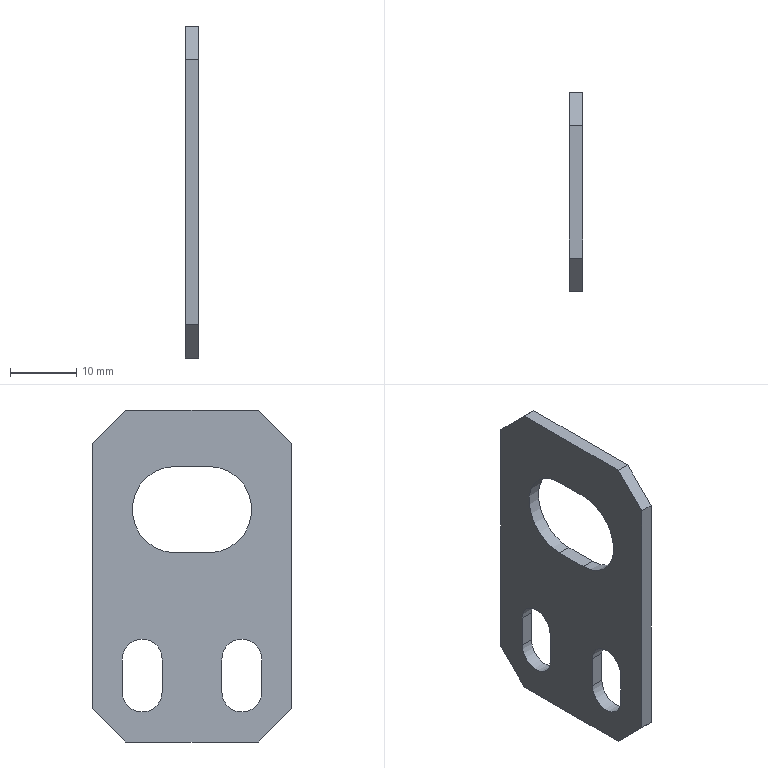Part | NX | features 5003_222_Bracket 2 | 1 solid | 22 faces | box 2 x 30 x 50 mm | volume 2271 mm3 | plane 16 | cylinder 6 | commonest cylinder face diameters 6 x4 13 x2
STEP:
#1=CARTESIAN_POINT('',(218.525,88.5,-44.5));
#2=VERTEX_POINT('',#1);
#3=CARTESIAN_POINT('',(218.525,88.5,-49.5));
#4=VERTEX_POINT('',#3);
#5=CARTESIAN_POINT('',(218.525,88.5,-44.5));
#6=DIRECTION('',(0.,0.,-1.));
#7=VECTOR('',#6,1000.);
#8=LINE('',#5,#7);
#9=EDGE_CURVE('',#2,#4,#8,.T.);
#10=ORIENTED_EDGE('',*,*,#9,.F.);
#11=CARTESIAN_POINT('',(218.525,82.5,-44.5));
#12=VERTEX_POINT('',#11);
#13=CARTESIAN_POINT('',(218.525,85.5,-44.5));
#14=DIRECTION('',(-1.,0.,0.));
#15=DIRECTION('',(0.,0.,-1.));
#16=AXIS2_PLACEMENT_3D('',#13,#14,#15);
#17=CIRCLE('',#16,3.);
#18=EDGE_CURVE('',#12,#2,#17,.T.);
#19=ORIENTED_EDGE('',*,*,#18,.F.);
#20=CARTESIAN_POINT('',(218.525,82.5,-49.5));
#21=VERTEX_POINT('',#20);
#22=CARTESIAN_POINT('',(218.525,82.5,-44.5));
#23=DIRECTION('',(0.,0.,1.));
#24=VECTOR('',#23,1000.);
#25=LINE('',#22,#24);
#26=EDGE_CURVE('',#21,#12,#25,.T.);
#27=ORIENTED_EDGE('',*,*,#26,.F.);
#28=CARTESIAN_POINT('',(218.525,85.5,-49.5));
#29=DIRECTION('',(-1.,0.,0.));
#30=DIRECTION('',(0.,0.,-1.));
#31=AXIS2_PLACEMENT_3D('',#28,#29,#30);
#32=CIRCLE('',#31,3.);
#33=EDGE_CURVE('',#4,#21,#32,.T.);
#34=ORIENTED_EDGE('',*,*,#33,.F.);
#35=EDGE_LOOP('',(#10,#19,#27,#34));
#36=FACE_BOUND('',#35,.T.);
#37=CARTESIAN_POINT('',(218.525,78.,-52.));
#38=VERTEX_POINT('',#37);
#39=CARTESIAN_POINT('',(218.525,78.,-12.));
#40=VERTEX_POINT('',#39);
#41=CARTESIAN_POINT('',(218.525,78.,-52.));
#42=DIRECTION('',(0.,0.,1.));
#43=VECTOR('',#42,1000.);
#44=LINE('',#41,#43);
#45=EDGE_CURVE('',#38,#40,#44,.T.);
#46=ORIENTED_EDGE('',*,*,#45,.T.);
#47=CARTESIAN_POINT('',(218.525,83.,-7.));
#48=VERTEX_POINT('',#47);
#49=CARTESIAN_POINT('',(218.525,78.,-12.));
#50=DIRECTION('',(0.,0.7071,0.7071));
#51=VECTOR('',#50,1000.);
#52=LINE('',#49,#51);
#53=EDGE_CURVE('',#40,#48,#52,.T.);
#54=ORIENTED_EDGE('',*,*,#53,.T.);
#55=CARTESIAN_POINT('',(218.525,103.,-7.));
#56=VERTEX_POINT('',#55);
#57=CARTESIAN_POINT('',(218.525,83.,-7.));
#58=DIRECTION('',(0.,1.,0.));
#59=VECTOR('',#58,1000.);
#60=LINE('',#57,#59);
#61=EDGE_CURVE('',#48,#56,#60,.T.);
#62=ORIENTED_EDGE('',*,*,#61,.T.);
#63=CARTESIAN_POINT('',(218.525,108.,-12.));
#64=VERTEX_POINT('',#63);
#65=CARTESIAN_POINT('',(218.525,103.,-7.));
#66=DIRECTION('',(0.,0.7071,-0.7071));
#67=VECTOR('',#66,1000.);
#68=LINE('',#65,#67);
#69=EDGE_CURVE('',#56,#64,#68,.T.);
#70=ORIENTED_EDGE('',*,*,#69,.T.);
#71=CARTESIAN_POINT('',(218.525,108.,-52.));
#72=VERTEX_POINT('',#71);
#73=CARTESIAN_POINT('',(218.525,108.,-12.));
#74=DIRECTION('',(0.,0.,-1.));
#75=VECTOR('',#74,1000.);
#76=LINE('',#73,#75);
#77=EDGE_CURVE('',#64,#72,#76,.T.);
#78=ORIENTED_EDGE('',*,*,#77,.T.);
#79=CARTESIAN_POINT('',(218.525,103.,-57.));
#80=VERTEX_POINT('',#79);
#81=CARTESIAN_POINT('',(218.525,108.,-52.));
#82=DIRECTION('',(0.,-0.7071,-0.7071));
#83=VECTOR('',#82,1000.);
#84=LINE('',#81,#83);
#85=EDGE_CURVE('',#72,#80,#84,.T.);
#86=ORIENTED_EDGE('',*,*,#85,.T.);
#87=CARTESIAN_POINT('',(218.525,83.,-57.));
#88=VERTEX_POINT('',#87);
#89=CARTESIAN_POINT('',(218.525,103.,-57.));
#90=DIRECTION('',(0.,-1.,0.));
#91=VECTOR('',#90,1000.);
#92=LINE('',#89,#91);
#93=EDGE_CURVE('',#80,#88,#92,.T.);
#94=ORIENTED_EDGE('',*,*,#93,.T.);
#95=CARTESIAN_POINT('',(218.525,83.,-57.));
#96=DIRECTION('',(0.,-0.7071,0.7071));
#97=VECTOR('',#96,1000.);
#98=LINE('',#95,#97);
#99=EDGE_CURVE('',#88,#38,#98,.T.);
#100=ORIENTED_EDGE('',*,*,#99,.T.);
#101=EDGE_LOOP('',(#46,#54,#62,#70,#78,#86,#94,#100));
#102=FACE_BOUND('',#101,.T.);
#103=CARTESIAN_POINT('',(218.525,90.5,-15.5));
#104=VERTEX_POINT('',#103);
#105=CARTESIAN_POINT('',(218.525,95.5,-15.5));
#106=VERTEX_POINT('',#105);
#107=CARTESIAN_POINT('',(218.525,90.5,-15.5));
#108=DIRECTION('',(0.,1.,0.));
#109=VECTOR('',#108,1000.);
#110=LINE('',#107,#109);
#111=EDGE_CURVE('',#104,#106,#110,.T.);
#112=ORIENTED_EDGE('',*,*,#111,.F.);
#113=CARTESIAN_POINT('',(218.525,90.5,-28.5));
#114=VERTEX_POINT('',#113);
#115=CARTESIAN_POINT('',(218.525,90.5,-22.));
#116=DIRECTION('',(-1.,0.,0.));
#117=DIRECTION('',(0.,0.,-1.));
#118=AXIS2_PLACEMENT_3D('',#115,#116,#117);
#119=CIRCLE('',#118,6.5);
#120=EDGE_CURVE('',#114,#104,#119,.T.);
#121=ORIENTED_EDGE('',*,*,#120,.F.);
#122=CARTESIAN_POINT('',(218.525,95.5,-28.5));
#123=VERTEX_POINT('',#122);
#124=CARTESIAN_POINT('',(218.525,90.5,-28.5));
#125=DIRECTION('',(0.,-1.,0.));
#126=VECTOR('',#125,1000.);
#127=LINE('',#124,#126);
#128=EDGE_CURVE('',#123,#114,#127,.T.);
#129=ORIENTED_EDGE('',*,*,#128,.F.);
#130=CARTESIAN_POINT('',(218.525,95.5,-22.));
#131=DIRECTION('',(-1.,0.,0.));
#132=DIRECTION('',(0.,0.,-1.));
#133=AXIS2_PLACEMENT_3D('',#130,#131,#132);
#134=CIRCLE('',#133,6.5);
#135=EDGE_CURVE('',#106,#123,#134,.T.);
#136=ORIENTED_EDGE('',*,*,#135,.F.);
#137=EDGE_LOOP('',(#112,#121,#129,#136));
#138=FACE_BOUND('',#137,.T.);
#139=CARTESIAN_POINT('',(218.525,97.5,-49.5));
#140=VERTEX_POINT('',#139);
#141=CARTESIAN_POINT('',(218.525,97.5,-44.5));
#142=VERTEX_POINT('',#141);
#143=CARTESIAN_POINT('',(218.525,97.5,-44.5));
#144=DIRECTION('',(0.,0.,1.));
#145=VECTOR('',#144,1000.);
#146=LINE('',#143,#145);
#147=EDGE_CURVE('',#140,#142,#146,.T.);
#148=ORIENTED_EDGE('',*,*,#147,.F.);
#149=CARTESIAN_POINT('',(218.525,103.5,-49.5));
#150=VERTEX_POINT('',#149);
#151=CARTESIAN_POINT('',(218.525,100.5,-49.5));
#152=DIRECTION('',(-1.,0.,0.));
#153=DIRECTION('',(0.,0.,-1.));
#154=AXIS2_PLACEMENT_3D('',#151,#152,#153);
#155=CIRCLE('',#154,3.);
#156=EDGE_CURVE('',#150,#140,#155,.T.);
#157=ORIENTED_EDGE('',*,*,#156,.F.);
#158=CARTESIAN_POINT('',(218.525,103.5,-44.5));
#159=VERTEX_POINT('',#158);
#160=CARTESIAN_POINT('',(218.525,103.5,-44.5));
#161=DIRECTION('',(0.,0.,-1.));
#162=VECTOR('',#161,1000.);
#163=LINE('',#160,#162);
#164=EDGE_CURVE('',#159,#150,#163,.T.);
#165=ORIENTED_EDGE('',*,*,#164,.F.);
#166=CARTESIAN_POINT('',(218.525,100.5,-44.5));
#167=DIRECTION('',(-1.,0.,0.));
#168=DIRECTION('',(0.,0.,-1.));
#169=AXIS2_PLACEMENT_3D('',#166,#167,#168);
#170=CIRCLE('',#169,3.);
#171=EDGE_CURVE('',#142,#159,#170,.T.);
#172=ORIENTED_EDGE('',*,*,#171,.F.);
#173=EDGE_LOOP('',(#148,#157,#165,#172));
#174=FACE_BOUND('',#173,.T.);
#175=CARTESIAN_POINT('',(218.525,108.,-32.));
#176=DIRECTION('',(-1.,0.,0.));
#177=DIRECTION('',(0.,0.,-1.));
#178=AXIS2_PLACEMENT_3D('',#175,#176,#177);
#179=PLANE('',#178);
#180=ADVANCED_FACE('',(#36,#102,#138,#174),#179,.T.);
#181=CARTESIAN_POINT('',(220.525,82.5,-44.5));
#182=VERTEX_POINT('',#181);
#183=CARTESIAN_POINT('',(220.525,88.5,-44.5));
#184=VERTEX_POINT('',#183);
#185=CARTESIAN_POINT('',(220.525,85.5,-44.5));
#186=DIRECTION('',(-1.,0.,0.));
#187=DIRECTION('',(0.,0.,-1.));
#188=AXIS2_PLACEMENT_3D('',#185,#186,#187);
#189=CIRCLE('',#188,3.);
#190=EDGE_CURVE('',#182,#184,#189,.T.);
#191=ORIENTED_EDGE('',*,*,#190,.T.);
#192=CARTESIAN_POINT('',(220.525,88.5,-49.5));
#193=VERTEX_POINT('',#192);
#194=CARTESIAN_POINT('',(220.525,88.5,-44.5));
#195=DIRECTION('',(0.,0.,-1.));
#196=VECTOR('',#195,1000.);
#197=LINE('',#194,#196);
#198=EDGE_CURVE('',#184,#193,#197,.T.);
#199=ORIENTED_EDGE('',*,*,#198,.T.);
#200=CARTESIAN_POINT('',(220.525,82.5,-49.5));
#201=VERTEX_POINT('',#200);
#202=CARTESIAN_POINT('',(220.525,85.5,-49.5));
#203=DIRECTION('',(-1.,0.,0.));
#204=DIRECTION('',(0.,0.,-1.));
#205=AXIS2_PLACEMENT_3D('',#202,#203,#204);
#206=CIRCLE('',#205,3.);
#207=EDGE_CURVE('',#193,#201,#206,.T.);
#208=ORIENTED_EDGE('',*,*,#207,.T.);
#209=CARTESIAN_POINT('',(220.525,82.5,-44.5));
#210=DIRECTION('',(0.,0.,1.));
#211=VECTOR('',#210,1000.);
#212=LINE('',#209,#211);
#213=EDGE_CURVE('',#201,#182,#212,.T.);
#214=ORIENTED_EDGE('',*,*,#213,.T.);
#215=EDGE_LOOP('',(#191,#199,#208,#214));
#216=FACE_BOUND('',#215,.T.);
#217=CARTESIAN_POINT('',(220.525,78.,-52.));
#218=VERTEX_POINT('',#217);
#219=CARTESIAN_POINT('',(220.525,78.,-12.));
#220=VERTEX_POINT('',#219);
#221=CARTESIAN_POINT('',(220.525,78.,-52.));
#222=DIRECTION('',(0.,0.,1.));
#223=VECTOR('',#222,1000.);
#224=LINE('',#221,#223);
#225=EDGE_CURVE('',#218,#220,#224,.T.);
#226=ORIENTED_EDGE('',*,*,#225,.F.);
#227=CARTESIAN_POINT('',(220.525,83.,-57.));
#228=VERTEX_POINT('',#227);
#229=CARTESIAN_POINT('',(220.525,83.,-57.));
#230=DIRECTION('',(0.,-0.7071,0.7071));
#231=VECTOR('',#230,1000.);
#232=LINE('',#229,#231);
#233=EDGE_CURVE('',#228,#218,#232,.T.);
#234=ORIENTED_EDGE('',*,*,#233,.F.);
#235=CARTESIAN_POINT('',(220.525,103.,-57.));
#236=VERTEX_POINT('',#235);
#237=CARTESIAN_POINT('',(220.525,103.,-57.));
#238=DIRECTION('',(0.,-1.,0.));
#239=VECTOR('',#238,1000.);
#240=LINE('',#237,#239);
#241=EDGE_CURVE('',#236,#228,#240,.T.);
#242=ORIENTED_EDGE('',*,*,#241,.F.);
#243=CARTESIAN_POINT('',(220.525,108.,-52.));
#244=VERTEX_POINT('',#243);
#245=CARTESIAN_POINT('',(220.525,108.,-52.));
#246=DIRECTION('',(0.,-0.7071,-0.7071));
#247=VECTOR('',#246,1000.);
#248=LINE('',#245,#247);
#249=EDGE_CURVE('',#244,#236,#248,.T.);
#250=ORIENTED_EDGE('',*,*,#249,.F.);
#251=CARTESIAN_POINT('',(220.525,108.,-12.));
#252=VERTEX_POINT('',#251);
#253=CARTESIAN_POINT('',(220.525,108.,-12.));
#254=DIRECTION('',(0.,0.,-1.));
#255=VECTOR('',#254,1000.);
#256=LINE('',#253,#255);
#257=EDGE_CURVE('',#252,#244,#256,.T.);
#258=ORIENTED_EDGE('',*,*,#257,.F.);
#259=CARTESIAN_POINT('',(220.525,103.,-7.));
#260=VERTEX_POINT('',#259);
#261=CARTESIAN_POINT('',(220.525,103.,-7.));
#262=DIRECTION('',(0.,0.7071,-0.7071));
#263=VECTOR('',#262,1000.);
#264=LINE('',#261,#263);
#265=EDGE_CURVE('',#260,#252,#264,.T.);
#266=ORIENTED_EDGE('',*,*,#265,.F.);
#267=CARTESIAN_POINT('',(220.525,83.,-7.));
#268=VERTEX_POINT('',#267);
#269=CARTESIAN_POINT('',(220.525,83.,-7.));
#270=DIRECTION('',(0.,1.,0.));
#271=VECTOR('',#270,1000.);
#272=LINE('',#269,#271);
#273=EDGE_CURVE('',#268,#260,#272,.T.);
#274=ORIENTED_EDGE('',*,*,#273,.F.);
#275=CARTESIAN_POINT('',(220.525,78.,-12.));
#276=DIRECTION('',(0.,0.7071,0.7071));
#277=VECTOR('',#276,1000.);
#278=LINE('',#275,#277);
#279=EDGE_CURVE('',#220,#268,#278,.T.);
#280=ORIENTED_EDGE('',*,*,#279,.F.);
#281=EDGE_LOOP('',(#226,#234,#242,#250,#258,#266,#274,#280));
#282=FACE_BOUND('',#281,.T.);
#283=CARTESIAN_POINT('',(220.525,90.5,-28.5));
#284=VERTEX_POINT('',#283);
#285=CARTESIAN_POINT('',(220.525,90.5,-15.5));
#286=VERTEX_POINT('',#285);
#287=CARTESIAN_POINT('',(220.525,90.5,-22.));
#288=DIRECTION('',(-1.,0.,0.));
#289=DIRECTION('',(0.,0.,-1.));
#290=AXIS2_PLACEMENT_3D('',#287,#288,#289);
#291=CIRCLE('',#290,6.5);
#292=EDGE_CURVE('',#284,#286,#291,.T.);
#293=ORIENTED_EDGE('',*,*,#292,.T.);
#294=CARTESIAN_POINT('',(220.525,95.5,-15.5));
#295=VERTEX_POINT('',#294);
#296=CARTESIAN_POINT('',(220.525,90.5,-15.5));
#297=DIRECTION('',(0.,1.,0.));
#298=VECTOR('',#297,1000.);
#299=LINE('',#296,#298);
#300=EDGE_CURVE('',#286,#295,#299,.T.);
#301=ORIENTED_EDGE('',*,*,#300,.T.);
#302=CARTESIAN_POINT('',(220.525,95.5,-28.5));
#303=VERTEX_POINT('',#302);
#304=CARTESIAN_POINT('',(220.525,95.5,-22.));
#305=DIRECTION('',(-1.,0.,0.));
#306=DIRECTION('',(0.,0.,-1.));
#307=AXIS2_PLACEMENT_3D('',#304,#305,#306);
#308=CIRCLE('',#307,6.5);
#309=EDGE_CURVE('',#295,#303,#308,.T.);
#310=ORIENTED_EDGE('',*,*,#309,.T.);
#311=CARTESIAN_POINT('',(220.525,90.5,-28.5));
#312=DIRECTION('',(0.,-1.,0.));
#313=VECTOR('',#312,1000.);
#314=LINE('',#311,#313);
#315=EDGE_CURVE('',#303,#284,#314,.T.);
#316=ORIENTED_EDGE('',*,*,#315,.T.);
#317=EDGE_LOOP('',(#293,#301,#310,#316));
#318=FACE_BOUND('',#317,.T.);
#319=CARTESIAN_POINT('',(220.525,103.5,-49.5));
#320=VERTEX_POINT('',#319);
#321=CARTESIAN_POINT('',(220.525,97.5,-49.5));
#322=VERTEX_POINT('',#321);
#323=CARTESIAN_POINT('',(220.525,100.5,-49.5));
#324=DIRECTION('',(-1.,0.,0.));
#325=DIRECTION('',(0.,0.,-1.));
#326=AXIS2_PLACEMENT_3D('',#323,#324,#325);
#327=CIRCLE('',#326,3.);
#328=EDGE_CURVE('',#320,#322,#327,.T.);
#329=ORIENTED_EDGE('',*,*,#328,.T.);
#330=CARTESIAN_POINT('',(220.525,97.5,-44.5));
#331=VERTEX_POINT('',#330);
#332=CARTESIAN_POINT('',(220.525,97.5,-44.5));
#333=DIRECTION('',(0.,0.,1.));
#334=VECTOR('',#333,1000.);
#335=LINE('',#332,#334);
#336=EDGE_CURVE('',#322,#331,#335,.T.);
#337=ORIENTED_EDGE('',*,*,#336,.T.);
#338=CARTESIAN_POINT('',(220.525,103.5,-44.5));
#339=VERTEX_POINT('',#338);
#340=CARTESIAN_POINT('',(220.525,100.5,-44.5));
#341=DIRECTION('',(-1.,0.,0.));
#342=DIRECTION('',(0.,0.,-1.));
#343=AXIS2_PLACEMENT_3D('',#340,#341,#342);
#344=CIRCLE('',#343,3.);
#345=EDGE_CURVE('',#331,#339,#344,.T.);
#346=ORIENTED_EDGE('',*,*,#345,.T.);
#347=CARTESIAN_POINT('',(220.525,103.5,-44.5));
#348=DIRECTION('',(0.,0.,-1.));
#349=VECTOR('',#348,1000.);
#350=LINE('',#347,#349);
#351=EDGE_CURVE('',#339,#320,#350,.T.);
#352=ORIENTED_EDGE('',*,*,#351,.T.);
#353=EDGE_LOOP('',(#329,#337,#346,#352));
#354=FACE_BOUND('',#353,.T.);
#355=CARTESIAN_POINT('',(220.525,108.,-32.));
#356=DIRECTION('',(-1.,0.,0.));
#357=DIRECTION('',(0.,0.,-1.));
#358=AXIS2_PLACEMENT_3D('',#355,#356,#357);
#359=PLANE('',#358);
#360=ADVANCED_FACE('',(#216,#282,#318,#354),#359,.F.);
#361=ORIENTED_EDGE('',*,*,#225,.T.);
#362=CARTESIAN_POINT('',(218.525,78.,-12.));
#363=DIRECTION('',(1.,0.,0.));
#364=VECTOR('',#363,1000.);
#365=LINE('',#362,#364);
#366=EDGE_CURVE('',#40,#220,#365,.T.);
#367=ORIENTED_EDGE('',*,*,#366,.F.);
#368=ORIENTED_EDGE('',*,*,#45,.F.);
#369=CARTESIAN_POINT('',(218.525,78.,-52.));
#370=DIRECTION('',(1.,0.,0.));
#371=VECTOR('',#370,1000.);
#372=LINE('',#369,#371);
#373=EDGE_CURVE('',#38,#218,#372,.T.);
#374=ORIENTED_EDGE('',*,*,#373,.T.);
#375=EDGE_LOOP('',(#361,#367,#368,#374));
#376=FACE_BOUND('',#375,.T.);
#377=CARTESIAN_POINT('',(218.525,78.,-52.));
#378=DIRECTION('',(0.,1.,0.));
#379=DIRECTION('',(0.,0.,-1.));
#380=AXIS2_PLACEMENT_3D('',#377,#378,#379);
#381=PLANE('',#380);
#382=ADVANCED_FACE('',(#376),#381,.F.);
#383=ORIENTED_EDGE('',*,*,#279,.T.);
#384=CARTESIAN_POINT('',(218.525,83.,-7.));
#385=DIRECTION('',(1.,0.,0.));
#386=VECTOR('',#385,1000.);
#387=LINE('',#384,#386);
#388=EDGE_CURVE('',#48,#268,#387,.T.);
#389=ORIENTED_EDGE('',*,*,#388,.F.);
#390=ORIENTED_EDGE('',*,*,#53,.F.);
#391=ORIENTED_EDGE('',*,*,#366,.T.);
#392=EDGE_LOOP('',(#383,#389,#390,#391));
#393=FACE_BOUND('',#392,.T.);
#394=CARTESIAN_POINT('',(218.525,78.,-12.));
#395=DIRECTION('',(0.,0.7071,-0.7071));
#396=DIRECTION('',(0.,-0.7071,-0.7071));
#397=AXIS2_PLACEMENT_3D('',#394,#395,#396);
#398=PLANE('',#397);
#399=ADVANCED_FACE('',(#393),#398,.F.);
#400=ORIENTED_EDGE('',*,*,#273,.T.);
#401=CARTESIAN_POINT('',(218.525,103.,-7.));
#402=DIRECTION('',(1.,0.,0.));
#403=VECTOR('',#402,1000.);
#404=LINE('',#401,#403);
#405=EDGE_CURVE('',#56,#260,#404,.T.);
#406=ORIENTED_EDGE('',*,*,#405,.F.);
#407=ORIENTED_EDGE('',*,*,#61,.F.);
#408=ORIENTED_EDGE('',*,*,#388,.T.);
#409=EDGE_LOOP('',(#400,#406,#407,#408));
#410=FACE_BOUND('',#409,.T.);
#411=CARTESIAN_POINT('',(218.525,83.,-7.));
#412=DIRECTION('',(0.,0.,-1.));
#413=DIRECTION('',(1.,0.,0.));
#414=AXIS2_PLACEMENT_3D('',#411,#412,#413);
#415=PLANE('',#414);
#416=ADVANCED_FACE('',(#410),#415,.F.);
#417=ORIENTED_EDGE('',*,*,#265,.T.);
#418=CARTESIAN_POINT('',(218.525,108.,-12.));
#419=DIRECTION('',(1.,0.,0.));
#420=VECTOR('',#419,1000.);
#421=LINE('',#418,#420);
#422=EDGE_CURVE('',#64,#252,#421,.T.);
#423=ORIENTED_EDGE('',*,*,#422,.F.);
#424=ORIENTED_EDGE('',*,*,#69,.F.);
#425=ORIENTED_EDGE('',*,*,#405,.T.);
#426=EDGE_LOOP('',(#417,#423,#424,#425));
#427=FACE_BOUND('',#426,.T.);
#428=CARTESIAN_POINT('',(218.525,103.,-7.));
#429=DIRECTION('',(0.,-0.7071,-0.7071));
#430=DIRECTION('',(0.,-0.7071,0.7071));
#431=AXIS2_PLACEMENT_3D('',#428,#429,#430);
#432=PLANE('',#431);
#433=ADVANCED_FACE('',(#427),#432,.F.);
#434=ORIENTED_EDGE('',*,*,#257,.T.);
#435=CARTESIAN_POINT('',(218.525,108.,-52.));
#436=DIRECTION('',(1.,0.,0.));
#437=VECTOR('',#436,1000.);
#438=LINE('',#435,#437);
#439=EDGE_CURVE('',#72,#244,#438,.T.);
#440=ORIENTED_EDGE('',*,*,#439,.F.);
#441=ORIENTED_EDGE('',*,*,#77,.F.);
#442=ORIENTED_EDGE('',*,*,#422,.T.);
#443=EDGE_LOOP('',(#434,#440,#441,#442));
#444=FACE_BOUND('',#443,.T.);
#445=CARTESIAN_POINT('',(218.525,108.,-12.));
#446=DIRECTION('',(0.,-1.,0.));
#447=DIRECTION('',(0.,0.,1.));
#448=AXIS2_PLACEMENT_3D('',#445,#446,#447);
#449=PLANE('',#448);
#450=ADVANCED_FACE('',(#444),#449,.F.);
#451=ORIENTED_EDGE('',*,*,#249,.T.);
#452=CARTESIAN_POINT('',(218.525,103.,-57.));
#453=DIRECTION('',(1.,0.,0.));
#454=VECTOR('',#453,1000.);
#455=LINE('',#452,#454);
#456=EDGE_CURVE('',#80,#236,#455,.T.);
#457=ORIENTED_EDGE('',*,*,#456,.F.);
#458=ORIENTED_EDGE('',*,*,#85,.F.);
#459=ORIENTED_EDGE('',*,*,#439,.T.);
#460=EDGE_LOOP('',(#451,#457,#458,#459));
#461=FACE_BOUND('',#460,.T.);
#462=CARTESIAN_POINT('',(218.525,108.,-52.));
#463=DIRECTION('',(0.,-0.7071,0.7071));
#464=DIRECTION('',(0.,0.7071,0.7071));
#465=AXIS2_PLACEMENT_3D('',#462,#463,#464);
#466=PLANE('',#465);
#467=ADVANCED_FACE('',(#461),#466,.F.);
#468=ORIENTED_EDGE('',*,*,#241,.T.);
#469=CARTESIAN_POINT('',(218.525,83.,-57.));
#470=DIRECTION('',(1.,0.,0.));
#471=VECTOR('',#470,1000.);
#472=LINE('',#469,#471);
#473=EDGE_CURVE('',#88,#228,#472,.T.);
#474=ORIENTED_EDGE('',*,*,#473,.F.);
#475=ORIENTED_EDGE('',*,*,#93,.F.);
#476=ORIENTED_EDGE('',*,*,#456,.T.);
#477=EDGE_LOOP('',(#468,#474,#475,#476));
#478=FACE_BOUND('',#477,.T.);
#479=CARTESIAN_POINT('',(218.525,103.,-57.));
#480=DIRECTION('',(0.,0.,1.));
#481=DIRECTION('',(-1.,0.,0.));
#482=AXIS2_PLACEMENT_3D('',#479,#480,#481);
#483=PLANE('',#482);
#484=ADVANCED_FACE('',(#478),#483,.F.);
#485=ORIENTED_EDGE('',*,*,#233,.T.);
#486=ORIENTED_EDGE('',*,*,#373,.F.);
#487=ORIENTED_EDGE('',*,*,#99,.F.);
#488=ORIENTED_EDGE('',*,*,#473,.T.);
#489=EDGE_LOOP('',(#485,#486,#487,#488));
#490=FACE_BOUND('',#489,.T.);
#491=CARTESIAN_POINT('',(218.525,83.,-57.));
#492=DIRECTION('',(0.,0.7071,0.7071));
#493=DIRECTION('',(0.,0.7071,-0.7071));
#494=AXIS2_PLACEMENT_3D('',#491,#492,#493);
#495=PLANE('',#494);
#496=ADVANCED_FACE('',(#490),#495,.F.);
#497=ORIENTED_EDGE('',*,*,#292,.F.);
#498=CARTESIAN_POINT('',(218.525,90.5,-28.5));
#499=DIRECTION('',(1.,0.,0.));
#500=VECTOR('',#499,1000.);
#501=LINE('',#498,#500);
#502=EDGE_CURVE('',#114,#284,#501,.T.);
#503=ORIENTED_EDGE('',*,*,#502,.F.);
#504=ORIENTED_EDGE('',*,*,#120,.T.);
#505=CARTESIAN_POINT('',(218.525,90.5,-15.5));
#506=DIRECTION('',(1.,0.,0.));
#507=VECTOR('',#506,1000.);
#508=LINE('',#505,#507);
#509=EDGE_CURVE('',#104,#286,#508,.T.);
#510=ORIENTED_EDGE('',*,*,#509,.T.);
#511=EDGE_LOOP('',(#497,#503,#504,#510));
#512=FACE_BOUND('',#511,.T.);
#513=CARTESIAN_POINT('',(218.525,90.5,-22.));
#514=DIRECTION('',(1.,0.,0.));
#515=DIRECTION('',(0.,0.,1.));
#516=AXIS2_PLACEMENT_3D('',#513,#514,#515);
#517=CYLINDRICAL_SURFACE('',#516,6.5);
#518=ADVANCED_FACE('',(#512),#517,.F.);
#519=ORIENTED_EDGE('',*,*,#300,.F.);
#520=ORIENTED_EDGE('',*,*,#509,.F.);
#521=ORIENTED_EDGE('',*,*,#111,.T.);
#522=CARTESIAN_POINT('',(218.525,95.5,-15.5));
#523=DIRECTION('',(1.,0.,0.));
#524=VECTOR('',#523,1000.);
#525=LINE('',#522,#524);
#526=EDGE_CURVE('',#106,#295,#525,.T.);
#527=ORIENTED_EDGE('',*,*,#526,.T.);
#528=EDGE_LOOP('',(#519,#520,#521,#527));
#529=FACE_BOUND('',#528,.T.);
#530=CARTESIAN_POINT('',(218.525,90.5,-15.5));
#531=DIRECTION('',(0.,0.,-1.));
#532=DIRECTION('',(1.,0.,0.));
#533=AXIS2_PLACEMENT_3D('',#530,#531,#532);
#534=PLANE('',#533);
#535=ADVANCED_FACE('',(#529),#534,.T.);
#536=ORIENTED_EDGE('',*,*,#309,.F.);
#537=ORIENTED_EDGE('',*,*,#526,.F.);
#538=ORIENTED_EDGE('',*,*,#135,.T.);
#539=CARTESIAN_POINT('',(218.525,95.5,-28.5));
#540=DIRECTION('',(1.,0.,0.));
#541=VECTOR('',#540,1000.);
#542=LINE('',#539,#541);
#543=EDGE_CURVE('',#123,#303,#542,.T.);
#544=ORIENTED_EDGE('',*,*,#543,.T.);
#545=EDGE_LOOP('',(#536,#537,#538,#544));
#546=FACE_BOUND('',#545,.T.);
#547=CARTESIAN_POINT('',(218.525,95.5,-22.));
#548=DIRECTION('',(1.,0.,0.));
#549=DIRECTION('',(0.,0.,1.));
#550=AXIS2_PLACEMENT_3D('',#547,#548,#549);
#551=CYLINDRICAL_SURFACE('',#550,6.5);
#552=ADVANCED_FACE('',(#546),#551,.F.);
#553=ORIENTED_EDGE('',*,*,#315,.F.);
#554=ORIENTED_EDGE('',*,*,#543,.F.);
#555=ORIENTED_EDGE('',*,*,#128,.T.);
#556=ORIENTED_EDGE('',*,*,#502,.T.);
#557=EDGE_LOOP('',(#553,#554,#555,#556));
#558=FACE_BOUND('',#557,.T.);
#559=CARTESIAN_POINT('',(218.525,90.5,-28.5));
#560=DIRECTION('',(0.,0.,1.));
#561=DIRECTION('',(-1.,0.,0.));
#562=AXIS2_PLACEMENT_3D('',#559,#560,#561);
#563=PLANE('',#562);
#564=ADVANCED_FACE('',(#558),#563,.T.);
#565=ORIENTED_EDGE('',*,*,#190,.F.);
#566=CARTESIAN_POINT('',(218.525,82.5,-44.5));
#567=DIRECTION('',(1.,0.,0.));
#568=VECTOR('',#567,1000.);
#569=LINE('',#566,#568);
#570=EDGE_CURVE('',#12,#182,#569,.T.);
#571=ORIENTED_EDGE('',*,*,#570,.F.);
#572=ORIENTED_EDGE('',*,*,#18,.T.);
#573=CARTESIAN_POINT('',(218.525,88.5,-44.5));
#574=DIRECTION('',(1.,0.,0.));
#575=VECTOR('',#574,1000.);
#576=LINE('',#573,#575);
#577=EDGE_CURVE('',#2,#184,#576,.T.);
#578=ORIENTED_EDGE('',*,*,#577,.T.);
#579=EDGE_LOOP('',(#565,#571,#572,#578));
#580=FACE_BOUND('',#579,.T.);
#581=CARTESIAN_POINT('',(218.525,85.5,-44.5));
#582=DIRECTION('',(1.,0.,0.));
#583=DIRECTION('',(0.,0.,1.));
#584=AXIS2_PLACEMENT_3D('',#581,#582,#583);
#585=CYLINDRICAL_SURFACE('',#584,3.);
#586=ADVANCED_FACE('',(#580),#585,.F.);
#587=ORIENTED_EDGE('',*,*,#198,.F.);
#588=ORIENTED_EDGE('',*,*,#577,.F.);
#589=ORIENTED_EDGE('',*,*,#9,.T.);
#590=CARTESIAN_POINT('',(218.525,88.5,-49.5));
#591=DIRECTION('',(1.,0.,0.));
#592=VECTOR('',#591,1000.);
#593=LINE('',#590,#592);
#594=EDGE_CURVE('',#4,#193,#593,.T.);
#595=ORIENTED_EDGE('',*,*,#594,.T.);
#596=EDGE_LOOP('',(#587,#588,#589,#595));
#597=FACE_BOUND('',#596,.T.);
#598=CARTESIAN_POINT('',(218.525,88.5,-44.5));
#599=DIRECTION('',(0.,-1.,0.));
#600=DIRECTION('',(0.,0.,1.));
#601=AXIS2_PLACEMENT_3D('',#598,#599,#600);
#602=PLANE('',#601);
#603=ADVANCED_FACE('',(#597),#602,.T.);
#604=ORIENTED_EDGE('',*,*,#207,.F.);
#605=ORIENTED_EDGE('',*,*,#594,.F.);
#606=ORIENTED_EDGE('',*,*,#33,.T.);
#607=CARTESIAN_POINT('',(218.525,82.5,-49.5));
#608=DIRECTION('',(1.,0.,0.));
#609=VECTOR('',#608,1000.);
#610=LINE('',#607,#609);
#611=EDGE_CURVE('',#21,#201,#610,.T.);
#612=ORIENTED_EDGE('',*,*,#611,.T.);
#613=EDGE_LOOP('',(#604,#605,#606,#612));
#614=FACE_BOUND('',#613,.T.);
#615=CARTESIAN_POINT('',(218.525,85.5,-49.5));
#616=DIRECTION('',(1.,0.,0.));
#617=DIRECTION('',(0.,0.,1.));
#618=AXIS2_PLACEMENT_3D('',#615,#616,#617);
#619=CYLINDRICAL_SURFACE('',#618,3.);
#620=ADVANCED_FACE('',(#614),#619,.F.);
#621=ORIENTED_EDGE('',*,*,#213,.F.);
#622=ORIENTED_EDGE('',*,*,#611,.F.);
#623=ORIENTED_EDGE('',*,*,#26,.T.);
#624=ORIENTED_EDGE('',*,*,#570,.T.);
#625=EDGE_LOOP('',(#621,#622,#623,#624));
#626=FACE_BOUND('',#625,.T.);
#627=CARTESIAN_POINT('',(218.525,82.5,-44.5));
#628=DIRECTION('',(0.,1.,0.));
#629=DIRECTION('',(0.,0.,-1.));
#630=AXIS2_PLACEMENT_3D('',#627,#628,#629);
#631=PLANE('',#630);
#632=ADVANCED_FACE('',(#626),#631,.T.);
#633=ORIENTED_EDGE('',*,*,#328,.F.);
#634=CARTESIAN_POINT('',(218.525,103.5,-49.5));
#635=DIRECTION('',(1.,0.,0.));
#636=VECTOR('',#635,1000.);
#637=LINE('',#634,#636);
#638=EDGE_CURVE('',#150,#320,#637,.T.);
#639=ORIENTED_EDGE('',*,*,#638,.F.);
#640=ORIENTED_EDGE('',*,*,#156,.T.);
#641=CARTESIAN_POINT('',(218.525,97.5,-49.5));
#642=DIRECTION('',(1.,0.,0.));
#643=VECTOR('',#642,1000.);
#644=LINE('',#641,#643);
#645=EDGE_CURVE('',#140,#322,#644,.T.);
#646=ORIENTED_EDGE('',*,*,#645,.T.);
#647=EDGE_LOOP('',(#633,#639,#640,#646));
#648=FACE_BOUND('',#647,.T.);
#649=CARTESIAN_POINT('',(218.525,100.5,-49.5));
#650=DIRECTION('',(1.,0.,0.));
#651=DIRECTION('',(0.,0.,1.));
#652=AXIS2_PLACEMENT_3D('',#649,#650,#651);
#653=CYLINDRICAL_SURFACE('',#652,3.);
#654=ADVANCED_FACE('',(#648),#653,.F.);
#655=ORIENTED_EDGE('',*,*,#336,.F.);
#656=ORIENTED_EDGE('',*,*,#645,.F.);
#657=ORIENTED_EDGE('',*,*,#147,.T.);
#658=CARTESIAN_POINT('',(218.525,97.5,-44.5));
#659=DIRECTION('',(1.,0.,0.));
#660=VECTOR('',#659,1000.);
#661=LINE('',#658,#660);
#662=EDGE_CURVE('',#142,#331,#661,.T.);
#663=ORIENTED_EDGE('',*,*,#662,.T.);
#664=EDGE_LOOP('',(#655,#656,#657,#663));
#665=FACE_BOUND('',#664,.T.);
#666=CARTESIAN_POINT('',(218.525,97.5,-44.5));
#667=DIRECTION('',(0.,1.,0.));
#668=DIRECTION('',(0.,0.,-1.));
#669=AXIS2_PLACEMENT_3D('',#666,#667,#668);
#670=PLANE('',#669);
#671=ADVANCED_FACE('',(#665),#670,.T.);
#672=ORIENTED_EDGE('',*,*,#345,.F.);
#673=ORIENTED_EDGE('',*,*,#662,.F.);
#674=ORIENTED_EDGE('',*,*,#171,.T.);
#675=CARTESIAN_POINT('',(218.525,103.5,-44.5));
#676=DIRECTION('',(1.,0.,0.));
#677=VECTOR('',#676,1000.);
#678=LINE('',#675,#677);
#679=EDGE_CURVE('',#159,#339,#678,.T.);
#680=ORIENTED_EDGE('',*,*,#679,.T.);
#681=EDGE_LOOP('',(#672,#673,#674,#680));
#682=FACE_BOUND('',#681,.T.);
#683=CARTESIAN_POINT('',(218.525,100.5,-44.5));
#684=DIRECTION('',(1.,0.,0.));
#685=DIRECTION('',(0.,0.,1.));
#686=AXIS2_PLACEMENT_3D('',#683,#684,#685);
#687=CYLINDRICAL_SURFACE('',#686,3.);
#688=ADVANCED_FACE('',(#682),#687,.F.);
#689=ORIENTED_EDGE('',*,*,#351,.F.);
#690=ORIENTED_EDGE('',*,*,#679,.F.);
#691=ORIENTED_EDGE('',*,*,#164,.T.);
#692=ORIENTED_EDGE('',*,*,#638,.T.);
#693=EDGE_LOOP('',(#689,#690,#691,#692));
#694=FACE_BOUND('',#693,.T.);
#695=CARTESIAN_POINT('',(218.525,103.5,-44.5));
#696=DIRECTION('',(0.,-1.,0.));
#697=DIRECTION('',(0.,0.,1.));
#698=AXIS2_PLACEMENT_3D('',#695,#696,#697);
#699=PLANE('',#698);
#700=ADVANCED_FACE('',(#694),#699,.T.);
#701=CLOSED_SHELL('',(#180,#360,#382,#399,#416,#433,#450,#467,#484,#496,#518,#535,#552,#564,#586,#603,#620,#632,#654,#671,#688,#700));
#702=MANIFOLD_SOLID_BREP('',#701);
#703=(LENGTH_UNIT()NAMED_UNIT(*)SI_UNIT(.MILLI.,.METRE.));
#704=UNCERTAINTY_MEASURE_WITH_UNIT(LENGTH_MEASURE(0.00001),#703,'','');
#705=(NAMED_UNIT(*)PLANE_ANGLE_UNIT()SI_UNIT($,.RADIAN.));
#706=(NAMED_UNIT(*)SI_UNIT($,.STERADIAN.)SOLID_ANGLE_UNIT());
#707=(GEOMETRIC_REPRESENTATION_CONTEXT(3)GLOBAL_UNCERTAINTY_ASSIGNED_CONTEXT((#704))GLOBAL_UNIT_ASSIGNED_CONTEXT((#703,#705,#706))REPRESENTATION_CONTEXT('',''));
#708=ADVANCED_BREP_SHAPE_REPRESENTATION('',(#702),#707);